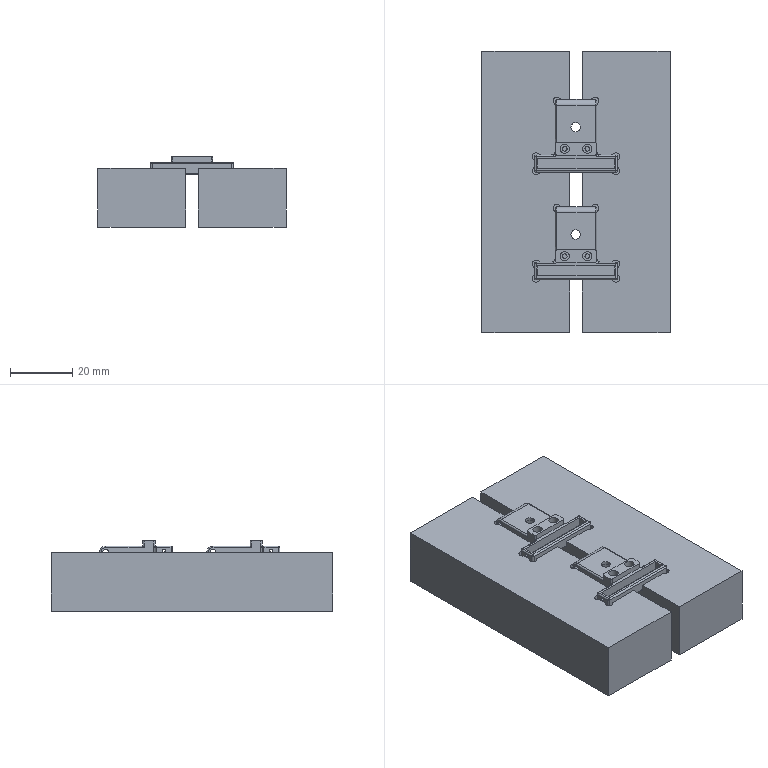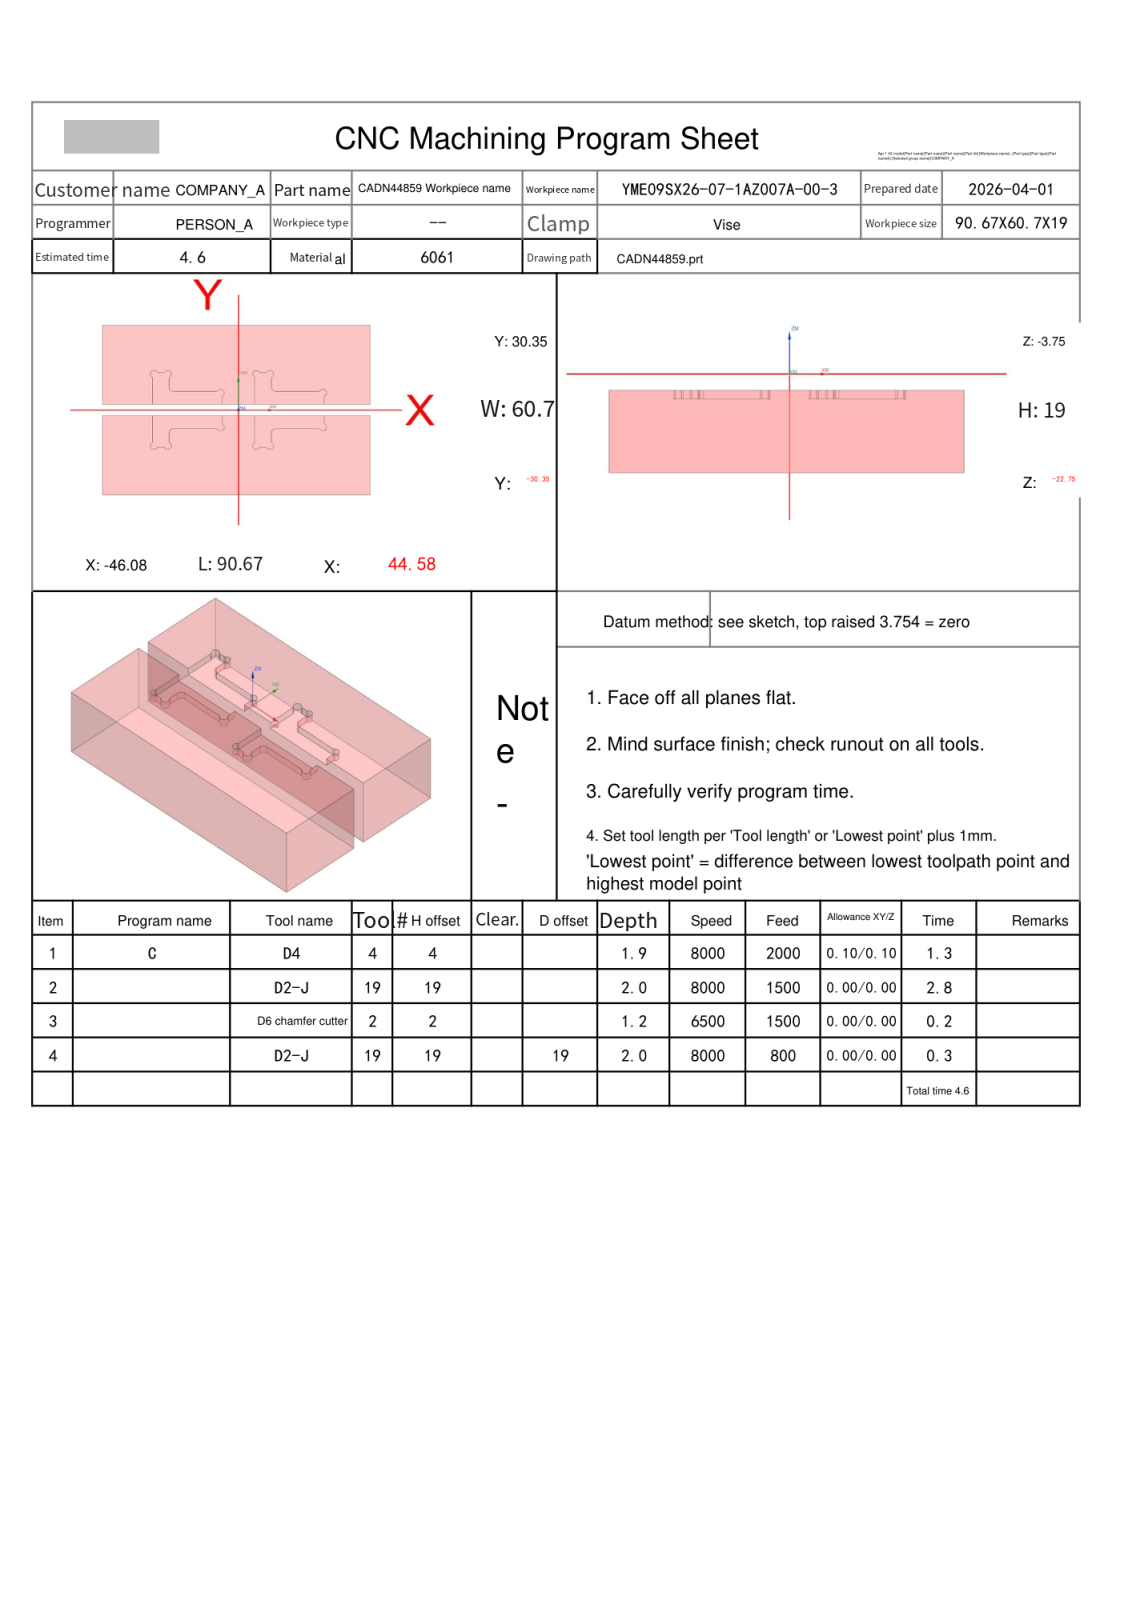NC program | NX | posted by the shop | part box 60.696 x 90.669 x 22.754 mm
Lines 7700 to 8014 of 8014:
N3 T02 M06
(D6 chamfer cutter  D=6. R=0. H=02 ce=0.00 di=0.00)
G00 G90 G54 X27.858 Y1.614 M03 S6500
G43 H02 Z46.246
M08
Z-3.641
G01 Z-4.953 F1500.
G03 X28.058 Y1.9 I-1.532 J1.286
G01 X28.087 Y1.946
X28.084 Y2.
Y4.698
G02 X28.727 Y5.929 I1.5 J0.0
G01 X28.801 Y6.008
X28.834 Y6.112
X28.819 Y6.219
X28.761 Y6.311
X28.67 Y6.369
X28.562 Y6.383
X28.459 Y6.35
X28.379 Y6.277
G02 X27.148 Y5.634 I-1.231 J.857
G01 X24.429
X22.617
X21.711
X18.992
X18.085
X16.273
X12.648
G02 X10.148 Y8.134 I0.0 J2.5
G01 Y11.412
G02 X10.791 Y12.643 I1.5 J0.0
G01 X10.864 Y12.723
X10.897 Y12.826
X10.883 Y12.933
X10.824 Y13.025
X10.733 Y13.083
X10.626 Y13.097
X10.522 Y13.064
X10.443 Y12.991
G02 X9.212 Y12.348 I-1.231 J.857
G01 X7.452
G02 X6.221 Y12.991 I0.0 J1.5
G01 X6.141 Y13.064
X6.038 Y13.097
X5.93 Y13.083
X5.839 Y13.025
X5.781 Y12.933
X5.766 Y12.826
X5.799 Y12.723
X5.873 Y12.643
G02 X6.516 Y11.412 I-.857 J-1.231
G01 Y2.
X6.513 Y1.946
X6.542 Y1.9
G03 X6.742 Y1.614 I1.732 J1.
G01 Z-3.641
G00 Z6.246
X-6.742
Z-3.641
G01 Z-4.953
G03 X-6.542 Y1.9 I-1.532 J1.286
G01 X-6.513 Y1.946
X-6.516 Y2.
Y4.698
G02 X-5.873 Y5.929 I1.5 J0.0
G01 X-5.799 Y6.008
X-5.766 Y6.112
X-5.781 Y6.219
X-5.839 Y6.311
X-5.93 Y6.369
X-6.038 Y6.383
X-6.141 Y6.35
X-6.221 Y6.277
G02 X-7.452 Y5.634 I-1.231 J.857
G01 X-21.952
G02 X-24.452 Y8.134 I0.0 J2.5
G01 Y11.412
G02 X-23.809 Y12.643 I1.5 J0.0
G01 X-23.736 Y12.723
X-23.703 Y12.826
X-23.717 Y12.933
X-23.776 Y13.025
X-23.867 Y13.083
X-23.974 Y13.097
X-24.078 Y13.064
X-24.157 Y12.991
G02 X-25.388 Y12.348 I-1.231 J.857
G01 X-27.148
G02 X-28.379 Y12.991 I0.0 J1.5
G01 X-28.459 Y13.064
X-28.562 Y13.097
X-28.67 Y13.083
X-28.761 Y13.025
X-28.819 Y12.933
X-28.834 Y12.826
X-28.801 Y12.723
X-28.727 Y12.643
G02 X-28.084 Y11.412 I-.857 J-1.231
G01 Y2.
X-28.087 Y1.946
X-28.058 Y1.9
G03 X-27.858 Y1.614 I1.732 J1.
G01 Z-3.641
G00 Z6.246
X6.742 Y-1.614
Z-3.641
G01 Z-4.953
G03 X6.542 Y-1.9 I1.532 J-1.286
G01 X6.513 Y-1.946
X6.516 Y-2.
Y-11.412
G02 X5.873 Y-12.643 I-1.5 J0.0
G01 X5.799 Y-12.723
X5.766 Y-12.826
X5.781 Y-12.933
X5.839 Y-13.025
X5.93 Y-13.083
X6.038 Y-13.097
X6.141 Y-13.064
X6.221 Y-12.991
G02 X7.452 Y-12.348 I1.231 J-.857
G01 X9.212
G02 X10.443 Y-12.991 I0.0 J-1.5
G01 X10.522 Y-13.064
X10.626 Y-13.097
X10.733 Y-13.083
X10.824 Y-13.025
X10.883 Y-12.933
X10.897 Y-12.826
X10.864 Y-12.723
X10.791 Y-12.643
G02 X10.148 Y-11.412 I.857 J1.231
G01 Y-8.134
G02 X12.648 Y-5.634 I2.5 J0.0
G01 X27.148
G02 X28.379 Y-6.277 I0.0 J-1.5
G01 X28.459 Y-6.35
X28.562 Y-6.383
X28.67 Y-6.369
X28.761 Y-6.311
X28.819 Y-6.219
X28.834 Y-6.112
X28.801 Y-6.008
X28.727 Y-5.929
G02 X28.084 Y-4.698 I.857 J1.231
G01 Y-2.
X28.087 Y-1.946
X28.058 Y-1.9
G03 X27.858 Y-1.614 I-1.732 J-1.
G01 Z-3.641
G00 Z6.246
X-27.858
Z-3.641
G01 Z-4.953
G03 X-28.058 Y-1.9 I1.532 J-1.286
G01 X-28.087 Y-1.946
X-28.084 Y-2.
Y-11.412
G02 X-28.727 Y-12.643 I-1.5 J0.0
G01 X-28.801 Y-12.723
X-28.834 Y-12.826
X-28.819 Y-12.933
X-28.761 Y-13.025
X-28.67 Y-13.083
X-28.562 Y-13.097
X-28.459 Y-13.064
X-28.379 Y-12.991
G02 X-27.148 Y-12.348 I1.231 J-.857
G01 X-25.388
G02 X-24.157 Y-12.991 I0.0 J-1.5
G01 X-24.078 Y-13.064
X-23.974 Y-13.097
X-23.867 Y-13.083
X-23.776 Y-13.025
X-23.717 Y-12.933
X-23.703 Y-12.826
X-23.736 Y-12.723
X-23.809 Y-12.643
G02 X-24.452 Y-11.412 I.857 J1.231
G01 Y-8.134
G02 X-21.952 Y-5.634 I2.5 J0.0
G01 X-7.452
G02 X-6.221 Y-6.277 I0.0 J-1.5
G01 X-6.141 Y-6.35
X-6.038 Y-6.383
X-5.93 Y-6.369
X-5.839 Y-6.311
X-5.781 Y-6.219
X-5.766 Y-6.112
X-5.799 Y-6.008
X-5.873 Y-5.929
G02 X-6.516 Y-4.698 I.857 J1.231
G01 Y-2.
X-6.513 Y-1.946
X-6.542 Y-1.9
G03 X-6.742 Y-1.614 I-1.732 J-1.
G01 Z-3.641
G00 Z46.246
G91 G28 Z0.0
M05
M09
G91 G28 Z0.0
M01
N4 T19 M06
(D2-J  D=2. R=0. H=19 ce=0.00 di=0.00)
G00 G90 G54 X-27.528 Y11.831 M03 S8000
G43 H19 Z6.246
M08
Z-4.754
G01 Z-5.754 F800.
G41 D19
X-27.727 Y11.81
G03 X-28.084 Y11.412 I.042 J-.398
G01 Y-11.412
G02 X-28.727 Y-12.643 I-1.5 J0.0
G03 X-28.834 Y-12.848 I.143 J-.205
X-28.584 Y-13.098 I.25 J0.0
X-28.379 Y-12.991 I0.0 J.25
G02 X-27.148 Y-12.348 I1.231 J-.857
G01 X-25.388
G02 X-24.157 Y-12.991 I0.0 J-1.5
G03 X-23.952 Y-13.098 I.205 J.143
X-23.702 Y-12.848 I0.0 J.25
X-23.809 Y-12.643 I-.25 J0.0
G02 X-24.452 Y-11.412 I.857 J1.231
G01 Y-8.134
G02 X-21.952 Y-5.634 I2.5 J0.0
G01 X-7.452
G02 X-6.221 Y-6.277 I0.0 J-1.5
G03 X-6.016 Y-6.384 I.205 J.143
X-5.766 Y-6.134 I0.0 J.25
X-5.873 Y-5.929 I-.25 J0.0
G02 X-6.516 Y-4.698 I.857 J1.231
G01 Y4.698
G02 X-5.873 Y5.929 I1.5 J0.0
G03 X-5.766 Y6.134 I-.143 J.205
X-6.016 Y6.384 I-.25 J0.0
X-6.221 Y6.277 I0.0 J-.25
G02 X-7.452 Y5.634 I-1.231 J.857
G01 X-21.952
G02 X-24.452 Y8.134 I0.0 J2.5
G01 Y11.412
G02 X-23.809 Y12.643 I1.5 J0.0
G03 X-23.702 Y12.848 I-.143 J.205
X-23.952 Y13.098 I-.25 J0.0
X-24.157 Y12.991 I0.0 J-.25
G02 X-25.388 Y12.348 I-1.231 J.857
G01 X-27.148
G02 X-28.379 Y12.991 I0.0 J1.5
G03 X-28.584 Y13.098 I-.205 J-.143
X-28.834 Y12.848 I0.0 J-.25
X-28.727 Y12.643 I.25 J0.0
G02 X-28.084 Y11.412 I-.857 J-1.231
G01 Y11.012
G03 X-27.684 Y10.612 I.4 J0.0
G01 G40 X-27.484
Z-4.754
G00 Z6.246
X7.072 Y11.831
Z-4.754
G01 Z-5.754
G41 D19
X6.873 Y11.81
G03 X6.516 Y11.412 I.042 J-.398
G01 Y-11.412
G02 X5.873 Y-12.643 I-1.5 J0.0
G03 X5.766 Y-12.848 I.143 J-.205
X6.016 Y-13.098 I.25 J0.0
X6.221 Y-12.991 I0.0 J.25
G02 X7.452 Y-12.348 I1.231 J-.857
G01 X9.212
G02 X10.443 Y-12.991 I0.0 J-1.5
G03 X10.648 Y-13.098 I.205 J.143
X10.898 Y-12.848 I0.0 J.25
X10.791 Y-12.643 I-.25 J0.0
G02 X10.148 Y-11.412 I.857 J1.231
G01 Y-8.134
G02 X12.648 Y-5.634 I2.5 J0.0
G01 X27.148
G02 X28.379 Y-6.277 I0.0 J-1.5
G03 X28.584 Y-6.384 I.205 J.143
X28.834 Y-6.134 I0.0 J.25
X28.727 Y-5.929 I-.25 J0.0
G02 X28.084 Y-4.698 I.857 J1.231
G01 Y4.698
G02 X28.727 Y5.929 I1.5 J0.0
G03 X28.834 Y6.134 I-.143 J.205
X28.584 Y6.384 I-.25 J0.0
X28.379 Y6.277 I0.0 J-.25
G02 X27.148 Y5.634 I-1.231 J.857
G01 X12.648
G02 X10.148 Y8.134 I0.0 J2.5
G01 Y11.412
G02 X10.791 Y12.643 I1.5 J0.0
G03 X10.898 Y12.848 I-.143 J.205
X10.648 Y13.098 I-.25 J0.0
X10.443 Y12.991 I0.0 J-.25
G02 X9.212 Y12.348 I-1.231 J.857
G01 X7.452
G02 X6.221 Y12.991 I0.0 J1.5
G03 X6.016 Y13.098 I-.205 J-.143
X5.766 Y12.848 I0.0 J-.25
X5.873 Y12.643 I.25 J0.0
G02 X6.516 Y11.412 I-.857 J-1.231
G01 Y11.012
G03 X6.916 Y10.612 I.4 J0.0
G01 G40 X7.116
Z-4.754
G00 Z6.246
M05
M09
G91 G28 Z0.0
G91 G28 Y0.0
M30
%